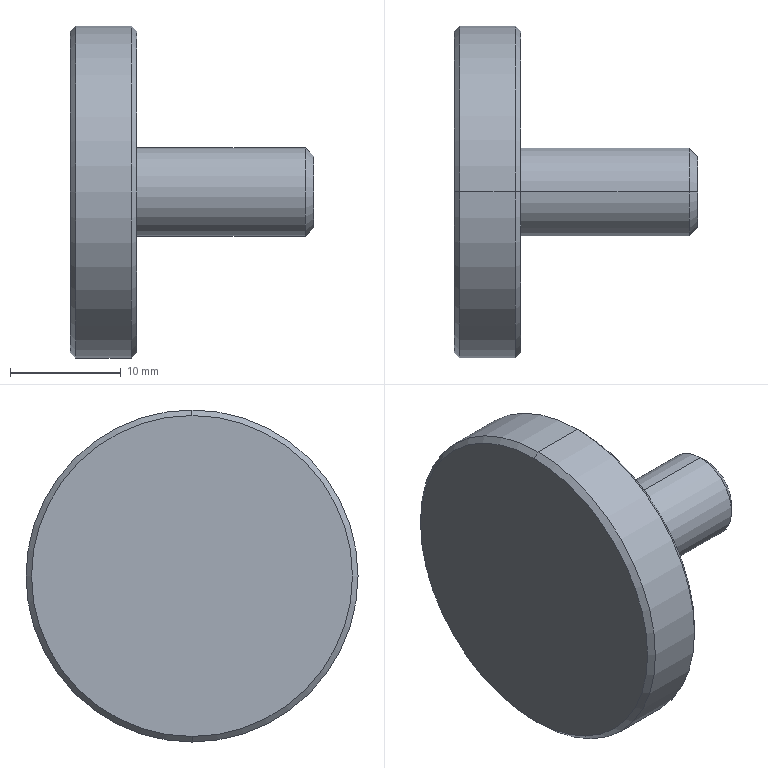Part | STEP file | 0217_007_NOOS8-16 | 1 solid | 13 faces | box 22 x 30 x 30 mm | volume 5015 mm3 | cone 6 | cylinder 4 | plane 3 | commonest cylinder face diameters 8 x2 30 x2
STEP:
#1=CARTESIAN_POINT('',(0.,0.,0.));
#2=DIRECTION('',(0.,0.,1.));
#3=DIRECTION('',(1.,0.,0.));
#4=AXIS2_PLACEMENT_3D('',#1,#2,#3);
#5=CARTESIAN_POINT('',(-6.,0.,14.5));
#6=VERTEX_POINT('',#5);
#7=CARTESIAN_POINT('',(-6.,0.,-14.5));
#8=VERTEX_POINT('',#7);
#9=CARTESIAN_POINT('',(-6.,0.,0.));
#10=DIRECTION('',(-1.,0.,0.));
#11=DIRECTION('',(0.,0.,-1.));
#12=AXIS2_PLACEMENT_3D('',#9,#10,#11);
#13=CIRCLE('',#12,14.5);
#14=CARTESIAN_POINT('',(-5.5,0.,0.));
#15=DIRECTION('',(1.,0.,0.));
#16=DIRECTION('',(0.,0.,-1.));
#17=AXIS2_PLACEMENT_3D('',#14,#15,#16);
#18=CONICAL_SURFACE('',#17,15.,0.7854);
#19=CARTESIAN_POINT('',(6.283,-0.5));
#20=DIRECTION('',(-1.,0.));
#21=VECTOR('',#20,1.);
#22=LINE('',#19,#21);
#23=(GEOMETRIC_REPRESENTATION_CONTEXT(2)PARAMETRIC_REPRESENTATION_CONTEXT()REPRESENTATION_CONTEXT('',''));
#24=DEFINITIONAL_REPRESENTATION('',(#22),#23);
#25=PCURVE('',#18,#24);
#26=CARTESIAN_POINT('',(-6.,7.25,0.));
#27=DIRECTION('',(-1.,0.,0.));
#28=DIRECTION('',(0.,0.,1.));
#29=AXIS2_PLACEMENT_3D('',#26,#27,#28);
#30=PLANE('',#29);
#31=CARTESIAN_POINT('',(0.,-7.25));
#32=DIRECTION('',(-1.,0.));
#33=AXIS2_PLACEMENT_2D('',#31,#32);
#34=CIRCLE('',#33,14.5);
#35=(GEOMETRIC_REPRESENTATION_CONTEXT(2)PARAMETRIC_REPRESENTATION_CONTEXT()REPRESENTATION_CONTEXT('',''));
#36=DEFINITIONAL_REPRESENTATION('',(#34),#35);
#37=PCURVE('',#30,#36);
#38=SURFACE_CURVE('',#13,(#25,#37),.PCURVE_S1.);
#39=EDGE_CURVE('',#6,#8,#38,.T.);
#40=ORIENTED_EDGE('',*,*,#39,.F.);
#41=CARTESIAN_POINT('',(-5.5,0.,15.));
#42=VERTEX_POINT('',#41);
#43=CARTESIAN_POINT('',(-5.5,0.,15.));
#44=DIRECTION('',(0.7071,0.,0.7071));
#45=VECTOR('',#44,1.);
#46=LINE('',#43,#45);
#47=CARTESIAN_POINT('',(3.142,0.));
#48=DIRECTION('',(0.,1.));
#49=VECTOR('',#48,1.);
#50=LINE('',#47,#49);
#51=(GEOMETRIC_REPRESENTATION_CONTEXT(2)PARAMETRIC_REPRESENTATION_CONTEXT()REPRESENTATION_CONTEXT('',''));
#52=DEFINITIONAL_REPRESENTATION('',(#50),#51);
#53=PCURVE('',#18,#52);
#54=CARTESIAN_POINT('',(-5.5,0.,0.));
#55=DIRECTION('',(1.,0.,0.));
#56=DIRECTION('',(0.,0.,-1.));
#57=AXIS2_PLACEMENT_3D('',#54,#55,#56);
#58=CONICAL_SURFACE('',#57,15.,0.7854);
#59=CARTESIAN_POINT('',(3.142,0.));
#60=DIRECTION('',(0.,1.));
#61=VECTOR('',#60,1.);
#62=LINE('',#59,#61);
#63=(GEOMETRIC_REPRESENTATION_CONTEXT(2)PARAMETRIC_REPRESENTATION_CONTEXT()REPRESENTATION_CONTEXT('',''));
#64=DEFINITIONAL_REPRESENTATION('',(#62),#63);
#65=PCURVE('',#58,#64);
#66=SURFACE_CURVE('',#46,(#53,#65),.PCURVE_S1.);
#67=EDGE_CURVE('',#6,#42,#66,.T.);
#68=ORIENTED_EDGE('',*,*,#67,.T.);
#69=CARTESIAN_POINT('',(-5.5,0.,-15.));
#70=VERTEX_POINT('',#69);
#71=CARTESIAN_POINT('',(-5.5,0.,0.));
#72=DIRECTION('',(-1.,0.,0.));
#73=DIRECTION('',(0.,1.,0.));
#74=AXIS2_PLACEMENT_3D('',#71,#72,#73);
#75=CIRCLE('',#74,15.);
#76=CARTESIAN_POINT('',(7.854,0.));
#77=DIRECTION('',(-1.,0.));
#78=VECTOR('',#77,1.);
#79=LINE('',#76,#78);
#80=(GEOMETRIC_REPRESENTATION_CONTEXT(2)PARAMETRIC_REPRESENTATION_CONTEXT()REPRESENTATION_CONTEXT('',''));
#81=DEFINITIONAL_REPRESENTATION('',(#79),#80);
#82=PCURVE('',#18,#81);
#83=CARTESIAN_POINT('',(-3.,0.,0.));
#84=DIRECTION('',(1.,0.,0.));
#85=DIRECTION('',(0.,0.,-1.));
#86=AXIS2_PLACEMENT_3D('',#83,#84,#85);
#87=CYLINDRICAL_SURFACE('',#86,15.);
#88=CARTESIAN_POINT('',(7.854,-2.5));
#89=DIRECTION('',(-1.,0.));
#90=VECTOR('',#89,1.);
#91=LINE('',#88,#90);
#92=(GEOMETRIC_REPRESENTATION_CONTEXT(2)PARAMETRIC_REPRESENTATION_CONTEXT()REPRESENTATION_CONTEXT('',''));
#93=DEFINITIONAL_REPRESENTATION('',(#91),#92);
#94=PCURVE('',#87,#93);
#95=SURFACE_CURVE('',#75,(#82,#94),.PCURVE_S1.);
#96=EDGE_CURVE('',#42,#70,#95,.T.);
#97=ORIENTED_EDGE('',*,*,#96,.T.);
#98=CARTESIAN_POINT('',(-5.5,0.,-15.));
#99=DIRECTION('',(0.7071,0.,-0.7071));
#100=VECTOR('',#99,1.);
#101=LINE('',#98,#100);
#102=CARTESIAN_POINT('',(0.,0.));
#103=DIRECTION('',(0.,1.));
#104=VECTOR('',#103,1.);
#105=LINE('',#102,#104);
#106=(GEOMETRIC_REPRESENTATION_CONTEXT(2)PARAMETRIC_REPRESENTATION_CONTEXT()REPRESENTATION_CONTEXT('',''));
#107=DEFINITIONAL_REPRESENTATION('',(#105),#106);
#108=PCURVE('',#18,#107);
#109=CARTESIAN_POINT('',(6.283,0.));
#110=DIRECTION('',(0.,1.));
#111=VECTOR('',#110,1.);
#112=LINE('',#109,#111);
#113=(GEOMETRIC_REPRESENTATION_CONTEXT(2)PARAMETRIC_REPRESENTATION_CONTEXT()REPRESENTATION_CONTEXT('',''));
#114=DEFINITIONAL_REPRESENTATION('',(#112),#113);
#115=PCURVE('',#58,#114);
#116=SURFACE_CURVE('',#101,(#108,#115),.PCURVE_S1.);
#117=EDGE_CURVE('',#8,#70,#116,.T.);
#118=ORIENTED_EDGE('',*,*,#117,.F.);
#119=EDGE_LOOP('',(#40,#68,#97,#118));
#120=FACE_BOUND('',#119,.T.);
#121=ADVANCED_FACE('',(#120),#18,.T.);
#122=ORIENTED_EDGE('',*,*,#96,.F.);
#123=CARTESIAN_POINT('',(-0.5,0.,15.));
#124=VERTEX_POINT('',#123);
#125=CARTESIAN_POINT('',(-3.,0.,15.));
#126=DIRECTION('',(1.,0.,0.));
#127=VECTOR('',#126,1.);
#128=LINE('',#125,#127);
#129=CARTESIAN_POINT('',(3.142,0.));
#130=DIRECTION('',(0.,1.));
#131=VECTOR('',#130,1.);
#132=LINE('',#129,#131);
#133=(GEOMETRIC_REPRESENTATION_CONTEXT(2)PARAMETRIC_REPRESENTATION_CONTEXT()REPRESENTATION_CONTEXT('',''));
#134=DEFINITIONAL_REPRESENTATION('',(#132),#133);
#135=PCURVE('',#87,#134);
#136=CARTESIAN_POINT('',(-3.,0.,0.));
#137=DIRECTION('',(1.,0.,0.));
#138=DIRECTION('',(0.,0.,-1.));
#139=AXIS2_PLACEMENT_3D('',#136,#137,#138);
#140=CYLINDRICAL_SURFACE('',#139,15.);
#141=CARTESIAN_POINT('',(3.142,0.));
#142=DIRECTION('',(0.,1.));
#143=VECTOR('',#142,1.);
#144=LINE('',#141,#143);
#145=(GEOMETRIC_REPRESENTATION_CONTEXT(2)PARAMETRIC_REPRESENTATION_CONTEXT()REPRESENTATION_CONTEXT('',''));
#146=DEFINITIONAL_REPRESENTATION('',(#144),#145);
#147=PCURVE('',#140,#146);
#148=SURFACE_CURVE('',#128,(#135,#147),.PCURVE_S1.);
#149=EDGE_CURVE('',#42,#124,#148,.T.);
#150=ORIENTED_EDGE('',*,*,#149,.T.);
#151=CARTESIAN_POINT('',(-0.5,0.,-15.));
#152=VERTEX_POINT('',#151);
#153=CARTESIAN_POINT('',(-0.5,0.,0.));
#154=DIRECTION('',(-1.,0.,0.));
#155=DIRECTION('',(0.,0.,-1.));
#156=AXIS2_PLACEMENT_3D('',#153,#154,#155);
#157=CIRCLE('',#156,15.);
#158=CARTESIAN_POINT('',(6.283,2.5));
#159=DIRECTION('',(-1.,0.));
#160=VECTOR('',#159,1.);
#161=LINE('',#158,#160);
#162=(GEOMETRIC_REPRESENTATION_CONTEXT(2)PARAMETRIC_REPRESENTATION_CONTEXT()REPRESENTATION_CONTEXT('',''));
#163=DEFINITIONAL_REPRESENTATION('',(#161),#162);
#164=PCURVE('',#87,#163);
#165=CARTESIAN_POINT('',(-0.5,0.,0.));
#166=DIRECTION('',(-1.,0.,0.));
#167=DIRECTION('',(0.,0.,1.));
#168=AXIS2_PLACEMENT_3D('',#165,#166,#167);
#169=CONICAL_SURFACE('',#168,15.,0.7854);
#170=CARTESIAN_POINT('',(-3.142,0.));
#171=DIRECTION('',(1.,0.));
#172=VECTOR('',#171,1.);
#173=LINE('',#170,#172);
#174=(GEOMETRIC_REPRESENTATION_CONTEXT(2)PARAMETRIC_REPRESENTATION_CONTEXT()REPRESENTATION_CONTEXT('',''));
#175=DEFINITIONAL_REPRESENTATION('',(#173),#174);
#176=PCURVE('',#169,#175);
#177=SURFACE_CURVE('',#157,(#164,#176),.PCURVE_S1.);
#178=EDGE_CURVE('',#124,#152,#177,.T.);
#179=ORIENTED_EDGE('',*,*,#178,.T.);
#180=CARTESIAN_POINT('',(-3.,0.,-15.));
#181=DIRECTION('',(1.,0.,0.));
#182=VECTOR('',#181,1.);
#183=LINE('',#180,#182);
#184=CARTESIAN_POINT('',(0.,0.));
#185=DIRECTION('',(0.,1.));
#186=VECTOR('',#185,1.);
#187=LINE('',#184,#186);
#188=(GEOMETRIC_REPRESENTATION_CONTEXT(2)PARAMETRIC_REPRESENTATION_CONTEXT()REPRESENTATION_CONTEXT('',''));
#189=DEFINITIONAL_REPRESENTATION('',(#187),#188);
#190=PCURVE('',#87,#189);
#191=CARTESIAN_POINT('',(6.283,0.));
#192=DIRECTION('',(0.,1.));
#193=VECTOR('',#192,1.);
#194=LINE('',#191,#193);
#195=(GEOMETRIC_REPRESENTATION_CONTEXT(2)PARAMETRIC_REPRESENTATION_CONTEXT()REPRESENTATION_CONTEXT('',''));
#196=DEFINITIONAL_REPRESENTATION('',(#194),#195);
#197=PCURVE('',#140,#196);
#198=SURFACE_CURVE('',#183,(#190,#197),.PCURVE_S1.);
#199=EDGE_CURVE('',#70,#152,#198,.T.);
#200=ORIENTED_EDGE('',*,*,#199,.F.);
#201=EDGE_LOOP('',(#122,#150,#179,#200));
#202=FACE_BOUND('',#201,.T.);
#203=ADVANCED_FACE('',(#202),#87,.T.);
#204=CARTESIAN_POINT('',(0.,0.,14.5));
#205=VERTEX_POINT('',#204);
#206=CARTESIAN_POINT('',(0.,0.,-14.5));
#207=VERTEX_POINT('',#206);
#208=CARTESIAN_POINT('',(0.,0.,0.));
#209=DIRECTION('',(-1.,0.,0.));
#210=DIRECTION('',(0.,0.,1.));
#211=AXIS2_PLACEMENT_3D('',#208,#209,#210);
#212=CIRCLE('',#211,14.5);
#213=CARTESIAN_POINT('',(0.,-0.5));
#214=DIRECTION('',(1.,0.));
#215=VECTOR('',#214,1.);
#216=LINE('',#213,#215);
#217=(GEOMETRIC_REPRESENTATION_CONTEXT(2)PARAMETRIC_REPRESENTATION_CONTEXT()REPRESENTATION_CONTEXT('',''));
#218=DEFINITIONAL_REPRESENTATION('',(#216),#217);
#219=PCURVE('',#169,#218);
#220=CARTESIAN_POINT('',(0.,7.25,0.));
#221=DIRECTION('',(1.,0.,0.));
#222=DIRECTION('',(0.,0.,-1.));
#223=AXIS2_PLACEMENT_3D('',#220,#221,#222);
#224=PLANE('',#223);
#225=CARTESIAN_POINT('',(-14.5,-7.25));
#226=CARTESIAN_POINT('',(-14.5,17.865));
#227=CARTESIAN_POINT('',(7.25,5.307));
#228=CARTESIAN_POINT('',(29.,-7.25));
#229=CARTESIAN_POINT('',(7.25,-19.807));
#230=CARTESIAN_POINT('',(-14.5,-32.365));
#231=CARTESIAN_POINT('',(-14.5,-7.25));
#232=(BOUNDED_CURVE()B_SPLINE_CURVE(2,(#225,#226,#227,#228,#229,#230,#231),.UNSPECIFIED.,.T.,.F.)B_SPLINE_CURVE_WITH_KNOTS((1,2,2,2,2,1),(-2.094,0.,2.094,4.189,6.283,8.378),.UNSPECIFIED.)CURVE()GEOMETRIC_REPRESENTATION_ITEM()RATIONAL_B_SPLINE_CURVE((1.,0.5,1.,0.5,1.,0.5,1.))REPRESENTATION_ITEM(''));
#233=(GEOMETRIC_REPRESENTATION_CONTEXT(2)PARAMETRIC_REPRESENTATION_CONTEXT()REPRESENTATION_CONTEXT('',''));
#234=DEFINITIONAL_REPRESENTATION('',(#232),#233);
#235=PCURVE('',#224,#234);
#236=SURFACE_CURVE('',#212,(#219,#235),.PCURVE_S1.);
#237=EDGE_CURVE('',#205,#207,#236,.T.);
#238=ORIENTED_EDGE('',*,*,#237,.T.);
#239=CARTESIAN_POINT('',(-0.5,0.,-15.));
#240=DIRECTION('',(-0.7071,0.,-0.7071));
#241=VECTOR('',#240,1.);
#242=LINE('',#239,#241);
#243=CARTESIAN_POINT('',(3.142,0.));
#244=DIRECTION('',(0.,1.));
#245=VECTOR('',#244,1.);
#246=LINE('',#243,#245);
#247=(GEOMETRIC_REPRESENTATION_CONTEXT(2)PARAMETRIC_REPRESENTATION_CONTEXT()REPRESENTATION_CONTEXT('',''));
#248=DEFINITIONAL_REPRESENTATION('',(#246),#247);
#249=PCURVE('',#169,#248);
#250=CARTESIAN_POINT('',(-0.5,0.,0.));
#251=DIRECTION('',(-1.,0.,0.));
#252=DIRECTION('',(0.,0.,1.));
#253=AXIS2_PLACEMENT_3D('',#250,#251,#252);
#254=CONICAL_SURFACE('',#253,15.,0.7854);
#255=CARTESIAN_POINT('',(3.142,0.));
#256=DIRECTION('',(0.,1.));
#257=VECTOR('',#256,1.);
#258=LINE('',#255,#257);
#259=(GEOMETRIC_REPRESENTATION_CONTEXT(2)PARAMETRIC_REPRESENTATION_CONTEXT()REPRESENTATION_CONTEXT('',''));
#260=DEFINITIONAL_REPRESENTATION('',(#258),#259);
#261=PCURVE('',#254,#260);
#262=SURFACE_CURVE('',#242,(#249,#261),.PCURVE_S1.);
#263=EDGE_CURVE('',#207,#152,#262,.T.);
#264=ORIENTED_EDGE('',*,*,#263,.T.);
#265=ORIENTED_EDGE('',*,*,#178,.F.);
#266=CARTESIAN_POINT('',(-0.5,0.,15.));
#267=DIRECTION('',(-0.7071,0.,0.7071));
#268=VECTOR('',#267,1.);
#269=LINE('',#266,#268);
#270=CARTESIAN_POINT('',(0.,0.));
#271=DIRECTION('',(0.,1.));
#272=VECTOR('',#271,1.);
#273=LINE('',#270,#272);
#274=(GEOMETRIC_REPRESENTATION_CONTEXT(2)PARAMETRIC_REPRESENTATION_CONTEXT()REPRESENTATION_CONTEXT('',''));
#275=DEFINITIONAL_REPRESENTATION('',(#273),#274);
#276=PCURVE('',#169,#275);
#277=CARTESIAN_POINT('',(6.283,0.));
#278=DIRECTION('',(0.,1.));
#279=VECTOR('',#278,1.);
#280=LINE('',#277,#279);
#281=(GEOMETRIC_REPRESENTATION_CONTEXT(2)PARAMETRIC_REPRESENTATION_CONTEXT()REPRESENTATION_CONTEXT('',''));
#282=DEFINITIONAL_REPRESENTATION('',(#280),#281);
#283=PCURVE('',#254,#282);
#284=SURFACE_CURVE('',#269,(#276,#283),.PCURVE_S1.);
#285=EDGE_CURVE('',#205,#124,#284,.T.);
#286=ORIENTED_EDGE('',*,*,#285,.F.);
#287=EDGE_LOOP('',(#238,#264,#265,#286));
#288=FACE_BOUND('',#287,.T.);
#289=ADVANCED_FACE('',(#288),#169,.T.);
#290=CARTESIAN_POINT('',(0.,0.,4.));
#291=VERTEX_POINT('',#290);
#292=CARTESIAN_POINT('',(0.,0.,-4.));
#293=VERTEX_POINT('',#292);
#294=CARTESIAN_POINT('',(0.,0.,0.));
#295=DIRECTION('',(-1.,0.,0.));
#296=DIRECTION('',(0.,0.,-1.));
#297=AXIS2_PLACEMENT_3D('',#294,#295,#296);
#298=CIRCLE('',#297,4.);
#299=CARTESIAN_POINT('',(7.617,0.,0.));
#300=DIRECTION('',(1.,0.,0.));
#301=DIRECTION('',(0.,0.,-1.));
#302=AXIS2_PLACEMENT_3D('',#299,#300,#301);
#303=CYLINDRICAL_SURFACE('',#302,4.);
#304=CARTESIAN_POINT('',(6.283,-7.617));
#305=DIRECTION('',(-1.,0.));
#306=VECTOR('',#305,1.);
#307=LINE('',#304,#306);
#308=(GEOMETRIC_REPRESENTATION_CONTEXT(2)PARAMETRIC_REPRESENTATION_CONTEXT()REPRESENTATION_CONTEXT('',''));
#309=DEFINITIONAL_REPRESENTATION('',(#307),#308);
#310=PCURVE('',#303,#309);
#311=CARTESIAN_POINT('',(4.,-7.25));
#312=CARTESIAN_POINT('',(4.,-14.178));
#313=CARTESIAN_POINT('',(-2.,-10.714));
#314=CARTESIAN_POINT('',(-8.,-7.25));
#315=CARTESIAN_POINT('',(-2.,-3.786));
#316=CARTESIAN_POINT('',(4.,-0.3218));
#317=CARTESIAN_POINT('',(4.,-7.25));
#318=(BOUNDED_CURVE()B_SPLINE_CURVE(2,(#311,#312,#313,#314,#315,#316,#317),.UNSPECIFIED.,.T.,.F.)B_SPLINE_CURVE_WITH_KNOTS((1,2,2,2,2,1),(-2.094,0.,2.094,4.189,6.283,8.378),.UNSPECIFIED.)CURVE()GEOMETRIC_REPRESENTATION_ITEM()RATIONAL_B_SPLINE_CURVE((1.,0.5,1.,0.5,1.,0.5,1.))REPRESENTATION_ITEM(''));
#319=(GEOMETRIC_REPRESENTATION_CONTEXT(2)PARAMETRIC_REPRESENTATION_CONTEXT()REPRESENTATION_CONTEXT('',''));
#320=DEFINITIONAL_REPRESENTATION('',(#318),#319);
#321=PCURVE('',#224,#320);
#322=SURFACE_CURVE('',#298,(#310,#321),.PCURVE_S1.);
#323=EDGE_CURVE('',#291,#293,#322,.T.);
#324=ORIENTED_EDGE('',*,*,#323,.F.);
#325=CARTESIAN_POINT('',(15.233,0.,4.));
#326=VERTEX_POINT('',#325);
#327=CARTESIAN_POINT('',(7.617,0.,4.));
#328=DIRECTION('',(1.,0.,0.));
#329=VECTOR('',#328,1.);
#330=LINE('',#327,#329);
#331=CARTESIAN_POINT('',(3.142,0.));
#332=DIRECTION('',(0.,1.));
#333=VECTOR('',#332,1.);
#334=LINE('',#331,#333);
#335=(GEOMETRIC_REPRESENTATION_CONTEXT(2)PARAMETRIC_REPRESENTATION_CONTEXT()REPRESENTATION_CONTEXT('',''));
#336=DEFINITIONAL_REPRESENTATION('',(#334),#335);
#337=PCURVE('',#303,#336);
#338=CARTESIAN_POINT('',(7.617,0.,0.));
#339=DIRECTION('',(1.,0.,0.));
#340=DIRECTION('',(0.,0.,-1.));
#341=AXIS2_PLACEMENT_3D('',#338,#339,#340);
#342=CYLINDRICAL_SURFACE('',#341,4.);
#343=CARTESIAN_POINT('',(3.142,0.));
#344=DIRECTION('',(0.,1.));
#345=VECTOR('',#344,1.);
#346=LINE('',#343,#345);
#347=(GEOMETRIC_REPRESENTATION_CONTEXT(2)PARAMETRIC_REPRESENTATION_CONTEXT()REPRESENTATION_CONTEXT('',''));
#348=DEFINITIONAL_REPRESENTATION('',(#346),#347);
#349=PCURVE('',#342,#348);
#350=SURFACE_CURVE('',#330,(#337,#349),.PCURVE_S1.);
#351=EDGE_CURVE('',#291,#326,#350,.T.);
#352=ORIENTED_EDGE('',*,*,#351,.T.);
#353=CARTESIAN_POINT('',(15.233,0.,-4.));
#354=VERTEX_POINT('',#353);
#355=CARTESIAN_POINT('',(15.233,0.,0.));
#356=DIRECTION('',(-1.,0.,0.));
#357=DIRECTION('',(0.,0.,-1.));
#358=AXIS2_PLACEMENT_3D('',#355,#356,#357);
#359=CIRCLE('',#358,4.);
#360=CARTESIAN_POINT('',(6.283,7.617));
#361=DIRECTION('',(-1.,0.));
#362=VECTOR('',#361,1.);
#363=LINE('',#360,#362);
#364=(GEOMETRIC_REPRESENTATION_CONTEXT(2)PARAMETRIC_REPRESENTATION_CONTEXT()REPRESENTATION_CONTEXT('',''));
#365=DEFINITIONAL_REPRESENTATION('',(#363),#364);
#366=PCURVE('',#303,#365);
#367=CARTESIAN_POINT('',(15.233,0.,0.));
#368=DIRECTION('',(-1.,0.,0.));
#369=DIRECTION('',(0.,0.,1.));
#370=AXIS2_PLACEMENT_3D('',#367,#368,#369);
#371=CONICAL_SURFACE('',#370,4.,0.7854);
#372=CARTESIAN_POINT('',(-3.142,0.));
#373=DIRECTION('',(1.,0.));
#374=VECTOR('',#373,1.);
#375=LINE('',#372,#374);
#376=(GEOMETRIC_REPRESENTATION_CONTEXT(2)PARAMETRIC_REPRESENTATION_CONTEXT()REPRESENTATION_CONTEXT('',''));
#377=DEFINITIONAL_REPRESENTATION('',(#375),#376);
#378=PCURVE('',#371,#377);
#379=SURFACE_CURVE('',#359,(#366,#378),.PCURVE_S1.);
#380=EDGE_CURVE('',#326,#354,#379,.T.);
#381=ORIENTED_EDGE('',*,*,#380,.T.);
#382=CARTESIAN_POINT('',(7.617,0.,-4.));
#383=DIRECTION('',(1.,0.,0.));
#384=VECTOR('',#383,1.);
#385=LINE('',#382,#384);
#386=CARTESIAN_POINT('',(0.,0.));
#387=DIRECTION('',(0.,1.));
#388=VECTOR('',#387,1.);
#389=LINE('',#386,#388);
#390=(GEOMETRIC_REPRESENTATION_CONTEXT(2)PARAMETRIC_REPRESENTATION_CONTEXT()REPRESENTATION_CONTEXT('',''));
#391=DEFINITIONAL_REPRESENTATION('',(#389),#390);
#392=PCURVE('',#303,#391);
#393=CARTESIAN_POINT('',(6.283,0.));
#394=DIRECTION('',(0.,1.));
#395=VECTOR('',#394,1.);
#396=LINE('',#393,#395);
#397=(GEOMETRIC_REPRESENTATION_CONTEXT(2)PARAMETRIC_REPRESENTATION_CONTEXT()REPRESENTATION_CONTEXT('',''));
#398=DEFINITIONAL_REPRESENTATION('',(#396),#397);
#399=PCURVE('',#342,#398);
#400=SURFACE_CURVE('',#385,(#392,#399),.PCURVE_S1.);
#401=EDGE_CURVE('',#293,#354,#400,.T.);
#402=ORIENTED_EDGE('',*,*,#401,.F.);
#403=EDGE_LOOP('',(#324,#352,#381,#402));
#404=FACE_BOUND('',#403,.T.);
#405=ADVANCED_FACE('',(#404),#303,.T.);
#406=CARTESIAN_POINT('',(16.,0.,3.233));
#407=VERTEX_POINT('',#406);
#408=CARTESIAN_POINT('',(16.,0.,-3.233));
#409=VERTEX_POINT('',#408);
#410=CARTESIAN_POINT('',(16.,0.,0.));
#411=DIRECTION('',(-1.,0.,0.));
#412=DIRECTION('',(0.,0.,1.));
#413=AXIS2_PLACEMENT_3D('',#410,#411,#412);
#414=CIRCLE('',#413,3.233);
#415=CARTESIAN_POINT('',(0.,-0.767));
#416=DIRECTION('',(1.,0.));
#417=VECTOR('',#416,1.);
#418=LINE('',#415,#417);
#419=(GEOMETRIC_REPRESENTATION_CONTEXT(2)PARAMETRIC_REPRESENTATION_CONTEXT()REPRESENTATION_CONTEXT('',''));
#420=DEFINITIONAL_REPRESENTATION('',(#418),#419);
#421=PCURVE('',#371,#420);
#422=CARTESIAN_POINT('',(16.,1.617,0.));
#423=DIRECTION('',(1.,0.,0.));
#424=DIRECTION('',(0.,0.,-1.));
#425=AXIS2_PLACEMENT_3D('',#422,#423,#424);
#426=PLANE('',#425);
#427=CARTESIAN_POINT('',(-3.233,-1.617));
#428=CARTESIAN_POINT('',(-3.233,3.983));
#429=CARTESIAN_POINT('',(1.616,1.183));
#430=CARTESIAN_POINT('',(6.466,-1.617));
#431=CARTESIAN_POINT('',(1.616,-4.416));
#432=CARTESIAN_POINT('',(-3.233,-7.216));
#433=CARTESIAN_POINT('',(-3.233,-1.617));
#434=(BOUNDED_CURVE()B_SPLINE_CURVE(2,(#427,#428,#429,#430,#431,#432,#433),.UNSPECIFIED.,.T.,.F.)B_SPLINE_CURVE_WITH_KNOTS((1,2,2,2,2,1),(-2.094,0.,2.094,4.189,6.283,8.378),.UNSPECIFIED.)CURVE()GEOMETRIC_REPRESENTATION_ITEM()RATIONAL_B_SPLINE_CURVE((1.,0.5,1.,0.5,1.,0.5,1.))REPRESENTATION_ITEM(''));
#435=(GEOMETRIC_REPRESENTATION_CONTEXT(2)PARAMETRIC_REPRESENTATION_CONTEXT()REPRESENTATION_CONTEXT('',''));
#436=DEFINITIONAL_REPRESENTATION('',(#434),#435);
#437=PCURVE('',#426,#436);
#438=SURFACE_CURVE('',#414,(#421,#437),.PCURVE_S1.);
#439=EDGE_CURVE('',#407,#409,#438,.T.);
#440=ORIENTED_EDGE('',*,*,#439,.T.);
#441=CARTESIAN_POINT('',(15.233,0.,-4.));
#442=DIRECTION('',(-0.7071,0.,-0.7071));
#443=VECTOR('',#442,1.);
#444=LINE('',#441,#443);
#445=CARTESIAN_POINT('',(3.142,0.));
#446=DIRECTION('',(0.,1.));
#447=VECTOR('',#446,1.);
#448=LINE('',#445,#447);
#449=(GEOMETRIC_REPRESENTATION_CONTEXT(2)PARAMETRIC_REPRESENTATION_CONTEXT()REPRESENTATION_CONTEXT('',''));
#450=DEFINITIONAL_REPRESENTATION('',(#448),#449);
#451=PCURVE('',#371,#450);
#452=CARTESIAN_POINT('',(15.233,0.,0.));
#453=DIRECTION('',(-1.,0.,0.));
#454=DIRECTION('',(0.,0.,1.));
#455=AXIS2_PLACEMENT_3D('',#452,#453,#454);
#456=CONICAL_SURFACE('',#455,4.,0.7854);
#457=CARTESIAN_POINT('',(3.142,0.));
#458=DIRECTION('',(0.,1.));
#459=VECTOR('',#458,1.);
#460=LINE('',#457,#459);
#461=(GEOMETRIC_REPRESENTATION_CONTEXT(2)PARAMETRIC_REPRESENTATION_CONTEXT()REPRESENTATION_CONTEXT('',''));
#462=DEFINITIONAL_REPRESENTATION('',(#460),#461);
#463=PCURVE('',#456,#462);
#464=SURFACE_CURVE('',#444,(#451,#463),.PCURVE_S1.);
#465=EDGE_CURVE('',#409,#354,#464,.T.);
#466=ORIENTED_EDGE('',*,*,#465,.T.);
#467=ORIENTED_EDGE('',*,*,#380,.F.);
#468=CARTESIAN_POINT('',(15.233,0.,4.));
#469=DIRECTION('',(-0.7071,0.,0.7071));
#470=VECTOR('',#469,1.);
#471=LINE('',#468,#470);
#472=CARTESIAN_POINT('',(0.,0.));
#473=DIRECTION('',(0.,1.));
#474=VECTOR('',#473,1.);
#475=LINE('',#472,#474);
#476=(GEOMETRIC_REPRESENTATION_CONTEXT(2)PARAMETRIC_REPRESENTATION_CONTEXT()REPRESENTATION_CONTEXT('',''));
#477=DEFINITIONAL_REPRESENTATION('',(#475),#476);
#478=PCURVE('',#371,#477);
#479=CARTESIAN_POINT('',(6.283,0.));
#480=DIRECTION('',(0.,1.));
#481=VECTOR('',#480,1.);
#482=LINE('',#479,#481);
#483=(GEOMETRIC_REPRESENTATION_CONTEXT(2)PARAMETRIC_REPRESENTATION_CONTEXT()REPRESENTATION_CONTEXT('',''));
#484=DEFINITIONAL_REPRESENTATION('',(#482),#483);
#485=PCURVE('',#456,#484);
#486=SURFACE_CURVE('',#471,(#478,#485),.PCURVE_S1.);
#487=EDGE_CURVE('',#407,#326,#486,.T.);
#488=ORIENTED_EDGE('',*,*,#487,.F.);
#489=EDGE_LOOP('',(#440,#466,#467,#488));
#490=FACE_BOUND('',#489,.T.);
#491=ADVANCED_FACE('',(#490),#371,.T.);
#492=CARTESIAN_POINT('',(-6.,0.,0.));
#493=DIRECTION('',(-1.,0.,0.));
#494=DIRECTION('',(0.,0.,-1.));
#495=AXIS2_PLACEMENT_3D('',#492,#493,#494);
#496=CIRCLE('',#495,14.5);
#497=CARTESIAN_POINT('',(0.,-7.25));
#498=DIRECTION('',(-1.,0.));
#499=AXIS2_PLACEMENT_2D('',#497,#498);
#500=CIRCLE('',#499,14.5);
#501=(GEOMETRIC_REPRESENTATION_CONTEXT(2)PARAMETRIC_REPRESENTATION_CONTEXT()REPRESENTATION_CONTEXT('',''));
#502=DEFINITIONAL_REPRESENTATION('',(#500),#501);
#503=PCURVE('',#30,#502);
#504=CARTESIAN_POINT('',(6.283,-0.5));
#505=DIRECTION('',(-1.,0.));
#506=VECTOR('',#505,1.);
#507=LINE('',#504,#506);
#508=(GEOMETRIC_REPRESENTATION_CONTEXT(2)PARAMETRIC_REPRESENTATION_CONTEXT()REPRESENTATION_CONTEXT('',''));
#509=DEFINITIONAL_REPRESENTATION('',(#507),#508);
#510=PCURVE('',#58,#509);
#511=SURFACE_CURVE('',#496,(#503,#510),.PCURVE_S1.);
#512=EDGE_CURVE('',#8,#6,#511,.T.);
#513=ORIENTED_EDGE('',*,*,#512,.T.);
#514=ORIENTED_EDGE('',*,*,#39,.T.);
#515=EDGE_LOOP('',(#513,#514));
#516=FACE_BOUND('',#515,.T.);
#517=ADVANCED_FACE('',(#516),#30,.T.);
#518=ORIENTED_EDGE('',*,*,#67,.F.);
#519=ORIENTED_EDGE('',*,*,#512,.F.);
#520=ORIENTED_EDGE('',*,*,#117,.T.);
#521=CARTESIAN_POINT('',(-5.5,0.,0.));
#522=DIRECTION('',(-1.,0.,0.));
#523=DIRECTION('',(0.,1.,0.));
#524=AXIS2_PLACEMENT_3D('',#521,#522,#523);
#525=CIRCLE('',#524,15.);
#526=CARTESIAN_POINT('',(7.854,0.));
#527=DIRECTION('',(-1.,0.));
#528=VECTOR('',#527,1.);
#529=LINE('',#526,#528);
#530=(GEOMETRIC_REPRESENTATION_CONTEXT(2)PARAMETRIC_REPRESENTATION_CONTEXT()REPRESENTATION_CONTEXT('',''));
#531=DEFINITIONAL_REPRESENTATION('',(#529),#530);
#532=PCURVE('',#58,#531);
#533=CARTESIAN_POINT('',(7.854,-2.5));
#534=DIRECTION('',(-1.,0.));
#535=VECTOR('',#534,1.);
#536=LINE('',#533,#535);
#537=(GEOMETRIC_REPRESENTATION_CONTEXT(2)PARAMETRIC_REPRESENTATION_CONTEXT()REPRESENTATION_CONTEXT('',''));
#538=DEFINITIONAL_REPRESENTATION('',(#536),#537);
#539=PCURVE('',#140,#538);
#540=SURFACE_CURVE('',#525,(#532,#539),.PCURVE_S1.);
#541=EDGE_CURVE('',#70,#42,#540,.T.);
#542=ORIENTED_EDGE('',*,*,#541,.T.);
#543=EDGE_LOOP('',(#518,#519,#520,#542));
#544=FACE_BOUND('',#543,.T.);
#545=ADVANCED_FACE('',(#544),#58,.T.);
#546=ORIENTED_EDGE('',*,*,#149,.F.);
#547=ORIENTED_EDGE('',*,*,#541,.F.);
#548=ORIENTED_EDGE('',*,*,#199,.T.);
#549=CARTESIAN_POINT('',(-0.5,0.,0.));
#550=DIRECTION('',(-1.,0.,0.));
#551=DIRECTION('',(0.,0.,-1.));
#552=AXIS2_PLACEMENT_3D('',#549,#550,#551);
#553=CIRCLE('',#552,15.);
#554=CARTESIAN_POINT('',(6.283,2.5));
#555=DIRECTION('',(-1.,0.));
#556=VECTOR('',#555,1.);
#557=LINE('',#554,#556);
#558=(GEOMETRIC_REPRESENTATION_CONTEXT(2)PARAMETRIC_REPRESENTATION_CONTEXT()REPRESENTATION_CONTEXT('',''));
#559=DEFINITIONAL_REPRESENTATION('',(#557),#558);
#560=PCURVE('',#140,#559);
#561=CARTESIAN_POINT('',(3.142,0.));
#562=DIRECTION('',(1.,0.));
#563=VECTOR('',#562,1.);
#564=LINE('',#561,#563);
#565=(GEOMETRIC_REPRESENTATION_CONTEXT(2)PARAMETRIC_REPRESENTATION_CONTEXT()REPRESENTATION_CONTEXT('',''));
#566=DEFINITIONAL_REPRESENTATION('',(#564),#565);
#567=PCURVE('',#254,#566);
#568=SURFACE_CURVE('',#553,(#560,#567),.PCURVE_S1.);
#569=EDGE_CURVE('',#152,#124,#568,.T.);
#570=ORIENTED_EDGE('',*,*,#569,.T.);
#571=EDGE_LOOP('',(#546,#547,#548,#570));
#572=FACE_BOUND('',#571,.T.);
#573=ADVANCED_FACE('',(#572),#140,.T.);
#574=ORIENTED_EDGE('',*,*,#263,.F.);
#575=CARTESIAN_POINT('',(0.,0.,0.));
#576=DIRECTION('',(-1.,0.,0.));
#577=DIRECTION('',(0.,0.,1.));
#578=AXIS2_PLACEMENT_3D('',#575,#576,#577);
#579=CIRCLE('',#578,14.5);
#580=CARTESIAN_POINT('',(0.,-0.5));
#581=DIRECTION('',(1.,0.));
#582=VECTOR('',#581,1.);
#583=LINE('',#580,#582);
#584=(GEOMETRIC_REPRESENTATION_CONTEXT(2)PARAMETRIC_REPRESENTATION_CONTEXT()REPRESENTATION_CONTEXT('',''));
#585=DEFINITIONAL_REPRESENTATION('',(#583),#584);
#586=PCURVE('',#254,#585);
#587=CARTESIAN_POINT('',(-14.5,-7.25));
#588=CARTESIAN_POINT('',(-14.5,17.865));
#589=CARTESIAN_POINT('',(7.25,5.307));
#590=CARTESIAN_POINT('',(29.,-7.25));
#591=CARTESIAN_POINT('',(7.25,-19.807));
#592=CARTESIAN_POINT('',(-14.5,-32.365));
#593=CARTESIAN_POINT('',(-14.5,-7.25));
#594=(BOUNDED_CURVE()B_SPLINE_CURVE(2,(#587,#588,#589,#590,#591,#592,#593),.UNSPECIFIED.,.T.,.F.)B_SPLINE_CURVE_WITH_KNOTS((1,2,2,2,2,1),(-2.094,0.,2.094,4.189,6.283,8.378),.UNSPECIFIED.)CURVE()GEOMETRIC_REPRESENTATION_ITEM()RATIONAL_B_SPLINE_CURVE((1.,0.5,1.,0.5,1.,0.5,1.))REPRESENTATION_ITEM(''));
#595=(GEOMETRIC_REPRESENTATION_CONTEXT(2)PARAMETRIC_REPRESENTATION_CONTEXT()REPRESENTATION_CONTEXT('',''));
#596=DEFINITIONAL_REPRESENTATION('',(#594),#595);
#597=PCURVE('',#224,#596);
#598=SURFACE_CURVE('',#579,(#586,#597),.PCURVE_S1.);
#599=EDGE_CURVE('',#207,#205,#598,.T.);
#600=ORIENTED_EDGE('',*,*,#599,.T.);
#601=ORIENTED_EDGE('',*,*,#285,.T.);
#602=ORIENTED_EDGE('',*,*,#569,.F.);
#603=EDGE_LOOP('',(#574,#600,#601,#602));
#604=FACE_BOUND('',#603,.T.);
#605=ADVANCED_FACE('',(#604),#254,.T.);
#606=ORIENTED_EDGE('',*,*,#237,.F.);
#607=ORIENTED_EDGE('',*,*,#599,.F.);
#608=EDGE_LOOP('',(#606,#607));
#609=FACE_BOUND('',#608,.T.);
#610=CARTESIAN_POINT('',(0.,0.,0.));
#611=DIRECTION('',(-1.,0.,0.));
#612=DIRECTION('',(0.,0.,-1.));
#613=AXIS2_PLACEMENT_3D('',#610,#611,#612);
#614=CIRCLE('',#613,4.);
#615=CARTESIAN_POINT('',(4.,-7.25));
#616=CARTESIAN_POINT('',(4.,-14.178));
#617=CARTESIAN_POINT('',(-2.,-10.714));
#618=CARTESIAN_POINT('',(-8.,-7.25));
#619=CARTESIAN_POINT('',(-2.,-3.786));
#620=CARTESIAN_POINT('',(4.,-0.3218));
#621=CARTESIAN_POINT('',(4.,-7.25));
#622=(BOUNDED_CURVE()B_SPLINE_CURVE(2,(#615,#616,#617,#618,#619,#620,#621),.UNSPECIFIED.,.T.,.F.)B_SPLINE_CURVE_WITH_KNOTS((1,2,2,2,2,1),(-2.094,0.,2.094,4.189,6.283,8.378),.UNSPECIFIED.)CURVE()GEOMETRIC_REPRESENTATION_ITEM()RATIONAL_B_SPLINE_CURVE((1.,0.5,1.,0.5,1.,0.5,1.))REPRESENTATION_ITEM(''));
#623=(GEOMETRIC_REPRESENTATION_CONTEXT(2)PARAMETRIC_REPRESENTATION_CONTEXT()REPRESENTATION_CONTEXT('',''));
#624=DEFINITIONAL_REPRESENTATION('',(#622),#623);
#625=PCURVE('',#224,#624);
#626=CARTESIAN_POINT('',(6.283,-7.617));
#627=DIRECTION('',(-1.,0.));
#628=VECTOR('',#627,1.);
#629=LINE('',#626,#628);
#630=(GEOMETRIC_REPRESENTATION_CONTEXT(2)PARAMETRIC_REPRESENTATION_CONTEXT()REPRESENTATION_CONTEXT('',''));
#631=DEFINITIONAL_REPRESENTATION('',(#629),#630);
#632=PCURVE('',#342,#631);
#633=SURFACE_CURVE('',#614,(#625,#632),.PCURVE_S1.);
#634=EDGE_CURVE('',#293,#291,#633,.T.);
#635=ORIENTED_EDGE('',*,*,#634,.T.);
#636=ORIENTED_EDGE('',*,*,#323,.T.);
#637=EDGE_LOOP('',(#635,#636));
#638=FACE_BOUND('',#637,.T.);
#639=ADVANCED_FACE('',(#609,#638),#224,.T.);
#640=ORIENTED_EDGE('',*,*,#351,.F.);
#641=ORIENTED_EDGE('',*,*,#634,.F.);
#642=ORIENTED_EDGE('',*,*,#401,.T.);
#643=CARTESIAN_POINT('',(15.233,0.,0.));
#644=DIRECTION('',(-1.,0.,0.));
#645=DIRECTION('',(0.,0.,-1.));
#646=AXIS2_PLACEMENT_3D('',#643,#644,#645);
#647=CIRCLE('',#646,4.);
#648=CARTESIAN_POINT('',(6.283,7.617));
#649=DIRECTION('',(-1.,0.));
#650=VECTOR('',#649,1.);
#651=LINE('',#648,#650);
#652=(GEOMETRIC_REPRESENTATION_CONTEXT(2)PARAMETRIC_REPRESENTATION_CONTEXT()REPRESENTATION_CONTEXT('',''));
#653=DEFINITIONAL_REPRESENTATION('',(#651),#652);
#654=PCURVE('',#342,#653);
#655=CARTESIAN_POINT('',(3.142,0.));
#656=DIRECTION('',(1.,0.));
#657=VECTOR('',#656,1.);
#658=LINE('',#655,#657);
#659=(GEOMETRIC_REPRESENTATION_CONTEXT(2)PARAMETRIC_REPRESENTATION_CONTEXT()REPRESENTATION_CONTEXT('',''));
#660=DEFINITIONAL_REPRESENTATION('',(#658),#659);
#661=PCURVE('',#456,#660);
#662=SURFACE_CURVE('',#647,(#654,#661),.PCURVE_S1.);
#663=EDGE_CURVE('',#354,#326,#662,.T.);
#664=ORIENTED_EDGE('',*,*,#663,.T.);
#665=EDGE_LOOP('',(#640,#641,#642,#664));
#666=FACE_BOUND('',#665,.T.);
#667=ADVANCED_FACE('',(#666),#342,.T.);
#668=ORIENTED_EDGE('',*,*,#465,.F.);
#669=CARTESIAN_POINT('',(16.,0.,0.));
#670=DIRECTION('',(-1.,0.,0.));
#671=DIRECTION('',(0.,0.,1.));
#672=AXIS2_PLACEMENT_3D('',#669,#670,#671);
#673=CIRCLE('',#672,3.233);
#674=CARTESIAN_POINT('',(0.,-0.767));
#675=DIRECTION('',(1.,0.));
#676=VECTOR('',#675,1.);
#677=LINE('',#674,#676);
#678=(GEOMETRIC_REPRESENTATION_CONTEXT(2)PARAMETRIC_REPRESENTATION_CONTEXT()REPRESENTATION_CONTEXT('',''));
#679=DEFINITIONAL_REPRESENTATION('',(#677),#678);
#680=PCURVE('',#456,#679);
#681=CARTESIAN_POINT('',(-3.233,-1.617));
#682=CARTESIAN_POINT('',(-3.233,3.983));
#683=CARTESIAN_POINT('',(1.616,1.183));
#684=CARTESIAN_POINT('',(6.466,-1.617));
#685=CARTESIAN_POINT('',(1.616,-4.416));
#686=CARTESIAN_POINT('',(-3.233,-7.216));
#687=CARTESIAN_POINT('',(-3.233,-1.617));
#688=(BOUNDED_CURVE()B_SPLINE_CURVE(2,(#681,#682,#683,#684,#685,#686,#687),.UNSPECIFIED.,.T.,.F.)B_SPLINE_CURVE_WITH_KNOTS((1,2,2,2,2,1),(-2.094,0.,2.094,4.189,6.283,8.378),.UNSPECIFIED.)CURVE()GEOMETRIC_REPRESENTATION_ITEM()RATIONAL_B_SPLINE_CURVE((1.,0.5,1.,0.5,1.,0.5,1.))REPRESENTATION_ITEM(''));
#689=(GEOMETRIC_REPRESENTATION_CONTEXT(2)PARAMETRIC_REPRESENTATION_CONTEXT()REPRESENTATION_CONTEXT('',''));
#690=DEFINITIONAL_REPRESENTATION('',(#688),#689);
#691=PCURVE('',#426,#690);
#692=SURFACE_CURVE('',#673,(#680,#691),.PCURVE_S1.);
#693=EDGE_CURVE('',#409,#407,#692,.T.);
#694=ORIENTED_EDGE('',*,*,#693,.T.);
#695=ORIENTED_EDGE('',*,*,#487,.T.);
#696=ORIENTED_EDGE('',*,*,#663,.F.);
#697=EDGE_LOOP('',(#668,#694,#695,#696));
#698=FACE_BOUND('',#697,.T.);
#699=ADVANCED_FACE('',(#698),#456,.T.);
#700=ORIENTED_EDGE('',*,*,#439,.F.);
#701=ORIENTED_EDGE('',*,*,#693,.F.);
#702=EDGE_LOOP('',(#700,#701));
#703=FACE_BOUND('',#702,.T.);
#704=ADVANCED_FACE('',(#703),#426,.T.);
#705=CLOSED_SHELL('',(#121,#203,#289,#405,#491,#517,#545,#573,#605,#639,#667,#699,#704));
#706=MANIFOLD_SOLID_BREP('',#705);
#707=(LENGTH_UNIT()NAMED_UNIT(*)SI_UNIT(.MILLI.,.METRE.));
#708=UNCERTAINTY_MEASURE_WITH_UNIT(LENGTH_MEASURE(0.0000001),#707,'','');
#709=(NAMED_UNIT(*)PLANE_ANGLE_UNIT()SI_UNIT($,.RADIAN.));
#710=(NAMED_UNIT(*)SI_UNIT($,.STERADIAN.)SOLID_ANGLE_UNIT());
#711=(GEOMETRIC_REPRESENTATION_CONTEXT(3)GLOBAL_UNCERTAINTY_ASSIGNED_CONTEXT((#708))GLOBAL_UNIT_ASSIGNED_CONTEXT((#707,#709,#710))REPRESENTATION_CONTEXT('',''));
#712=ADVANCED_BREP_SHAPE_REPRESENTATION('',(#4,#706),#711);